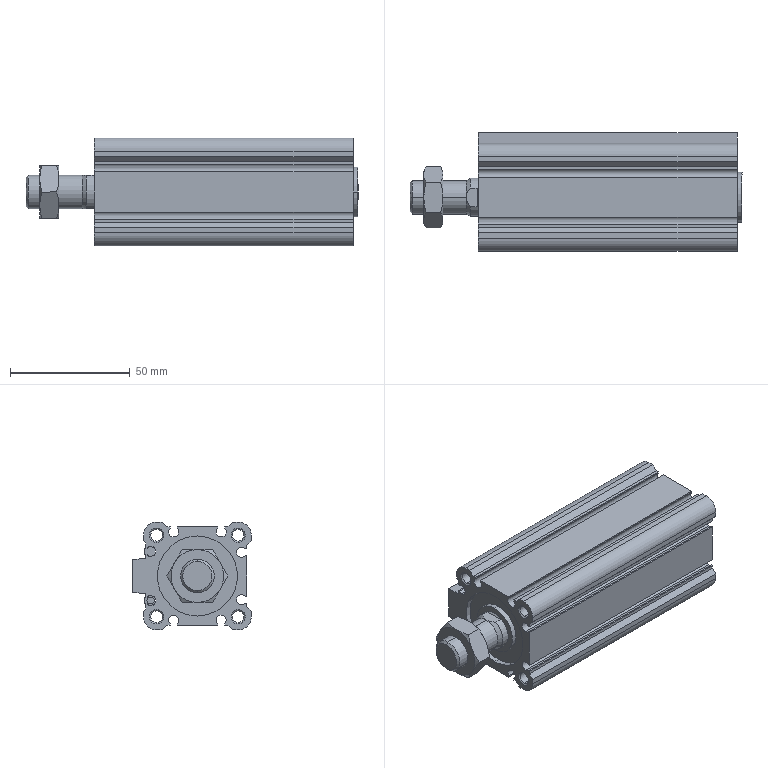Part | SolidWorks | 5 solids | 252 faces | box 138.5 x 49.5 x 45 mm | volume 140577 mm3 | plane 118 | cylinder 94 | cone 40 | commonest cylinder face diameters 4.26 x18 4.917 x16 0.6 x8 6 x8 4 x6 2 x4